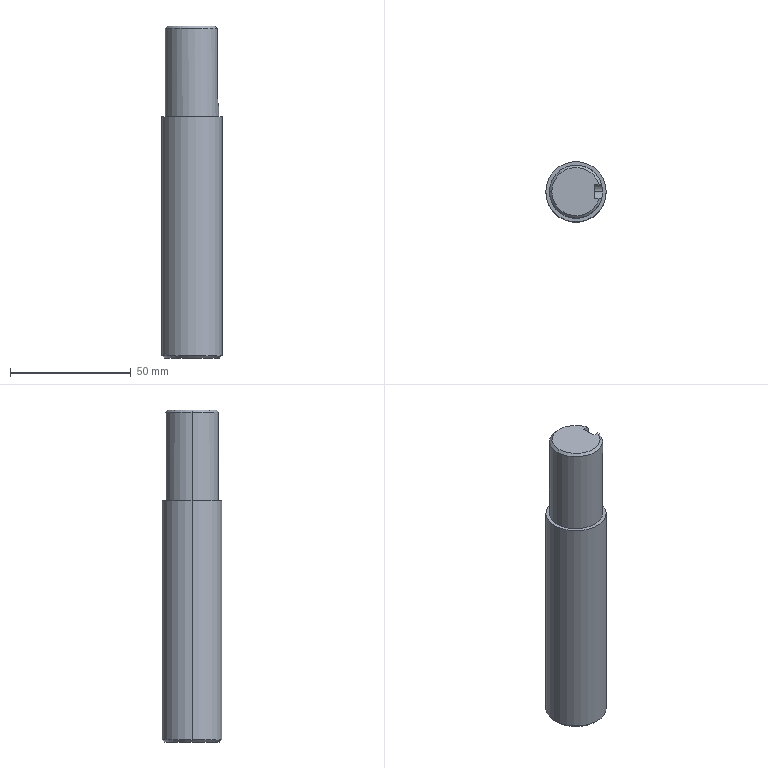Part | SolidWorks | features BaseBody 1 | 1 solid | 16 faces | box 25 x 25 x 137.5 mm | volume 62620 mm3 | cylinder 6 | plane 6 | cone 4 | commonest cylinder face diameters 6 x2 22 x2 25 x2
STEP:
#1=CARTESIAN_POINT('',(-12.5,0.,100.));
#2=VERTEX_POINT('',#1);
#3=CARTESIAN_POINT('',(12.5,0.,100.));
#4=VERTEX_POINT('',#3);
#5=CARTESIAN_POINT('',(0.,0.,100.));
#6=DIRECTION('',(0.,0.,-1.));
#7=DIRECTION('',(-1.,0.,0.));
#8=AXIS2_PLACEMENT_3D('',#5,#6,#7);
#9=CIRCLE('',#8,12.5);
#10=EDGE_CURVE('',#2,#4,#9,.T.);
#11=ORIENTED_EDGE('',*,*,#10,.T.);
#12=CARTESIAN_POINT('',(12.5,0.,1.));
#13=VERTEX_POINT('',#12);
#14=CARTESIAN_POINT('',(12.5,0.,100.));
#15=DIRECTION('',(0.,0.,-1.));
#16=VECTOR('',#15,1000.);
#17=LINE('',#14,#16);
#18=EDGE_CURVE('',#4,#13,#17,.T.);
#19=ORIENTED_EDGE('',*,*,#18,.T.);
#20=CARTESIAN_POINT('',(-12.5,0.,1.));
#21=VERTEX_POINT('',#20);
#22=CARTESIAN_POINT('',(0.,0.,1.));
#23=DIRECTION('',(0.,0.,1.));
#24=DIRECTION('',(-1.,0.,0.));
#25=AXIS2_PLACEMENT_3D('',#22,#23,#24);
#26=CIRCLE('',#25,12.5);
#27=EDGE_CURVE('',#13,#21,#26,.T.);
#28=ORIENTED_EDGE('',*,*,#27,.T.);
#29=CARTESIAN_POINT('',(-12.5,0.,100.));
#30=DIRECTION('',(0.,0.,-1.));
#31=VECTOR('',#30,1000.);
#32=LINE('',#29,#31);
#33=EDGE_CURVE('',#2,#21,#32,.T.);
#34=ORIENTED_EDGE('',*,*,#33,.F.);
#35=EDGE_LOOP('',(#11,#19,#28,#34));
#36=FACE_OUTER_BOUND('',#35,.T.);
#37=CARTESIAN_POINT('',(0.,0.,100.));
#38=DIRECTION('',(0.,0.,-1.));
#39=DIRECTION('',(-1.,0.,0.));
#40=AXIS2_PLACEMENT_3D('',#37,#38,#39);
#41=CYLINDRICAL_SURFACE('',#40,12.5);
#42=ADVANCED_FACE('',(#36),#41,.T.);
#43=CARTESIAN_POINT('',(11.5,0.,0.));
#44=VERTEX_POINT('',#43);
#45=CARTESIAN_POINT('',(-11.5,0.,0.));
#46=VERTEX_POINT('',#45);
#47=CARTESIAN_POINT('',(0.,0.,0.));
#48=DIRECTION('',(0.,0.,1.));
#49=DIRECTION('',(1.,0.,0.));
#50=AXIS2_PLACEMENT_3D('',#47,#48,#49);
#51=CIRCLE('',#50,11.5);
#52=EDGE_CURVE('',#44,#46,#51,.T.);
#53=ORIENTED_EDGE('',*,*,#52,.T.);
#54=CARTESIAN_POINT('',(-12.5,0.,1.));
#55=DIRECTION('',(-0.7071,0.,0.7071));
#56=VECTOR('',#55,1000.);
#57=LINE('',#54,#56);
#58=EDGE_CURVE('',#46,#21,#57,.T.);
#59=ORIENTED_EDGE('',*,*,#58,.T.);
#60=ORIENTED_EDGE('',*,*,#27,.F.);
#61=CARTESIAN_POINT('',(12.5,0.,1.));
#62=DIRECTION('',(0.7071,0.,0.7071));
#63=VECTOR('',#62,1000.);
#64=LINE('',#61,#63);
#65=EDGE_CURVE('',#44,#13,#64,.T.);
#66=ORIENTED_EDGE('',*,*,#65,.F.);
#67=EDGE_LOOP('',(#53,#59,#60,#66));
#68=FACE_OUTER_BOUND('',#67,.T.);
#69=CARTESIAN_POINT('',(0.,0.,1.));
#70=DIRECTION('',(0.,0.,1.));
#71=DIRECTION('',(1.,0.,0.));
#72=AXIS2_PLACEMENT_3D('',#69,#70,#71);
#73=CONICAL_SURFACE('',#72,12.5,0.7854);
#74=ADVANCED_FACE('',(#68),#73,.T.);
#75=CARTESIAN_POINT('',(10.583,3.,107.5));
#76=VERTEX_POINT('',#75);
#77=CARTESIAN_POINT('',(11.,0.,104.5));
#78=VERTEX_POINT('',#77);
#79=CARTESIAN_POINT('',(10.583,3.,107.5));
#80=CARTESIAN_POINT('',(10.583,3.,107.301));
#81=CARTESIAN_POINT('',(10.589,2.98,107.105));
#82=CARTESIAN_POINT('',(10.61,2.904,106.721));
#83=CARTESIAN_POINT('',(10.626,2.846,106.53));
#84=CARTESIAN_POINT('',(10.665,2.695,106.167));
#85=CARTESIAN_POINT('',(10.688,2.603,105.995));
#86=CARTESIAN_POINT('',(10.739,2.385,105.67));
#87=CARTESIAN_POINT('',(10.766,2.259,105.517));
#88=CARTESIAN_POINT('',(10.82,1.984,105.242));
#89=CARTESIAN_POINT('',(10.847,1.834,105.118));
#90=CARTESIAN_POINT('',(10.898,1.507,104.898));
#91=CARTESIAN_POINT('',(10.92,1.334,104.806));
#92=CARTESIAN_POINT('',(10.958,0.9736,104.656));
#93=CARTESIAN_POINT('',(10.974,0.784,104.597));
#94=CARTESIAN_POINT('',(10.995,0.3957,104.52));
#95=CARTESIAN_POINT('',(11.,0.1991,104.5));
#96=CARTESIAN_POINT('',(11.,0.,104.5));
#97=B_SPLINE_CURVE_WITH_KNOTS('',3,(#79,#80,#81,#82,#83,#84,#85,#86,#87,#88,#89,#90,#91,#92,#93,#94,#95,#96),.UNSPECIFIED.,.F.,.F.,(4,2,2,2,2,2,2,2,4),(0.,0.0005886,0.001177,0.001766,0.002354,0.002943,0.003532,0.00412,0.004709),.UNSPECIFIED.);
#98=EDGE_CURVE('',#76,#78,#97,.T.);
#99=ORIENTED_EDGE('',*,*,#98,.T.);
#100=CARTESIAN_POINT('',(11.,0.,100.));
#101=VERTEX_POINT('',#100);
#102=CARTESIAN_POINT('',(11.,0.,137.5));
#103=DIRECTION('',(0.,0.,-1.));
#104=VECTOR('',#103,1000.);
#105=LINE('',#102,#104);
#106=EDGE_CURVE('',#78,#101,#105,.T.);
#107=ORIENTED_EDGE('',*,*,#106,.T.);
#108=CARTESIAN_POINT('',(-11.,0.,100.));
#109=VERTEX_POINT('',#108);
#110=CARTESIAN_POINT('',(0.,0.,100.));
#111=DIRECTION('',(0.,0.,-1.));
#112=DIRECTION('',(-1.,0.,0.));
#113=AXIS2_PLACEMENT_3D('',#110,#111,#112);
#114=CIRCLE('',#113,11.);
#115=EDGE_CURVE('',#109,#101,#114,.T.);
#116=ORIENTED_EDGE('',*,*,#115,.F.);
#117=CARTESIAN_POINT('',(-11.,0.,136.5));
#118=VERTEX_POINT('',#117);
#119=CARTESIAN_POINT('',(-11.,0.,137.5));
#120=DIRECTION('',(0.,0.,-1.));
#121=VECTOR('',#120,1000.);
#122=LINE('',#119,#121);
#123=EDGE_CURVE('',#118,#109,#122,.T.);
#124=ORIENTED_EDGE('',*,*,#123,.F.);
#125=CARTESIAN_POINT('',(10.583,3.,136.5));
#126=VERTEX_POINT('',#125);
#127=CARTESIAN_POINT('',(0.,0.,136.5));
#128=DIRECTION('',(0.,0.,-1.));
#129=DIRECTION('',(-1.,0.,0.));
#130=AXIS2_PLACEMENT_3D('',#127,#128,#129);
#131=CIRCLE('',#130,11.);
#132=EDGE_CURVE('',#118,#126,#131,.T.);
#133=ORIENTED_EDGE('',*,*,#132,.T.);
#134=CARTESIAN_POINT('',(10.583,3.,137.5));
#135=DIRECTION('',(0.,0.,-1.));
#136=VECTOR('',#135,1000.);
#137=LINE('',#134,#136);
#138=EDGE_CURVE('',#126,#76,#137,.T.);
#139=ORIENTED_EDGE('',*,*,#138,.T.);
#140=EDGE_LOOP('',(#99,#107,#116,#124,#133,#139));
#141=FACE_OUTER_BOUND('',#140,.T.);
#142=CARTESIAN_POINT('',(0.,0.,137.5));
#143=DIRECTION('',(0.,0.,-1.));
#144=DIRECTION('',(-1.,0.,0.));
#145=AXIS2_PLACEMENT_3D('',#142,#143,#144);
#146=CYLINDRICAL_SURFACE('',#145,11.);
#147=ADVANCED_FACE('',(#141),#146,.T.);
#148=CARTESIAN_POINT('',(9.539,-3.,137.5));
#149=VERTEX_POINT('',#148);
#150=CARTESIAN_POINT('',(-10.,0.,137.5));
#151=VERTEX_POINT('',#150);
#152=CARTESIAN_POINT('',(0.,0.,137.5));
#153=DIRECTION('',(0.,0.,-1.));
#154=DIRECTION('',(-1.,0.,0.));
#155=AXIS2_PLACEMENT_3D('',#152,#153,#154);
#156=CIRCLE('',#155,10.);
#157=EDGE_CURVE('',#149,#151,#156,.T.);
#158=ORIENTED_EDGE('',*,*,#157,.T.);
#159=CARTESIAN_POINT('',(-11.,0.,136.5));
#160=DIRECTION('',(-0.7071,0.,-0.7071));
#161=VECTOR('',#160,1000.);
#162=LINE('',#159,#161);
#163=EDGE_CURVE('',#151,#118,#162,.T.);
#164=ORIENTED_EDGE('',*,*,#163,.T.);
#165=CARTESIAN_POINT('',(10.583,-3.,136.5));
#166=VERTEX_POINT('',#165);
#167=CARTESIAN_POINT('',(0.,0.,136.5));
#168=DIRECTION('',(0.,0.,-1.));
#169=DIRECTION('',(-1.,0.,0.));
#170=AXIS2_PLACEMENT_3D('',#167,#168,#169);
#171=CIRCLE('',#170,11.);
#172=EDGE_CURVE('',#166,#118,#171,.T.);
#173=ORIENTED_EDGE('',*,*,#172,.F.);
#174=CARTESIAN_POINT('',(10.583,-3.,136.5));
#175=CARTESIAN_POINT('',(10.236,-3.,136.834));
#176=CARTESIAN_POINT('',(9.888,-3.,137.167));
#177=CARTESIAN_POINT('',(9.539,-3.,137.5));
#178=B_SPLINE_CURVE_WITH_KNOTS('',3,(#174,#175,#176,#177),.UNSPECIFIED.,.F.,.F.,(4,4),(0.,0.001445),.UNSPECIFIED.);
#179=EDGE_CURVE('',#166,#149,#178,.T.);
#180=ORIENTED_EDGE('',*,*,#179,.T.);
#181=EDGE_LOOP('',(#158,#164,#173,#180));
#182=FACE_OUTER_BOUND('',#181,.T.);
#183=CARTESIAN_POINT('',(0.,0.,136.5));
#184=DIRECTION('',(0.,0.,-1.));
#185=DIRECTION('',(-1.,0.,0.));
#186=AXIS2_PLACEMENT_3D('',#183,#184,#185);
#187=CONICAL_SURFACE('',#186,11.,0.7854);
#188=ADVANCED_FACE('',(#182),#187,.T.);
#189=CARTESIAN_POINT('',(7.5,0.,104.5));
#190=VERTEX_POINT('',#189);
#191=CARTESIAN_POINT('',(7.5,3.,107.5));
#192=VERTEX_POINT('',#191);
#193=CARTESIAN_POINT('',(7.5,0.,107.5));
#194=DIRECTION('',(1.,0.,0.));
#195=DIRECTION('',(0.,0.,-1.));
#196=AXIS2_PLACEMENT_3D('',#193,#194,#195);
#197=CIRCLE('',#196,3.);
#198=EDGE_CURVE('',#190,#192,#197,.T.);
#199=ORIENTED_EDGE('',*,*,#198,.F.);
#200=CARTESIAN_POINT('',(7.5,0.,104.5));
#201=DIRECTION('',(1.,0.,0.));
#202=VECTOR('',#201,1000.);
#203=LINE('',#200,#202);
#204=EDGE_CURVE('',#190,#78,#203,.T.);
#205=ORIENTED_EDGE('',*,*,#204,.T.);
#206=ORIENTED_EDGE('',*,*,#98,.F.);
#207=CARTESIAN_POINT('',(7.5,3.,107.5));
#208=DIRECTION('',(-1.,0.,0.));
#209=VECTOR('',#208,1000.);
#210=LINE('',#207,#209);
#211=EDGE_CURVE('',#76,#192,#210,.T.);
#212=ORIENTED_EDGE('',*,*,#211,.T.);
#213=EDGE_LOOP('',(#199,#205,#206,#212));
#214=FACE_OUTER_BOUND('',#213,.T.);
#215=CARTESIAN_POINT('',(7.5,0.,107.5));
#216=DIRECTION('',(1.,0.,0.));
#217=DIRECTION('',(0.,0.,-1.));
#218=AXIS2_PLACEMENT_3D('',#215,#216,#217);
#219=CYLINDRICAL_SURFACE('',#218,3.);
#220=ADVANCED_FACE('',(#214),#219,.F.);
#221=ORIENTED_EDGE('',*,*,#18,.F.);
#222=CARTESIAN_POINT('',(0.,0.,100.));
#223=DIRECTION('',(0.,0.,-1.));
#224=DIRECTION('',(-1.,0.,0.));
#225=AXIS2_PLACEMENT_3D('',#222,#223,#224);
#226=CIRCLE('',#225,12.5);
#227=EDGE_CURVE('',#4,#2,#226,.T.);
#228=ORIENTED_EDGE('',*,*,#227,.T.);
#229=ORIENTED_EDGE('',*,*,#33,.T.);
#230=CARTESIAN_POINT('',(0.,0.,1.));
#231=DIRECTION('',(0.,0.,1.));
#232=DIRECTION('',(-1.,0.,0.));
#233=AXIS2_PLACEMENT_3D('',#230,#231,#232);
#234=CIRCLE('',#233,12.5);
#235=EDGE_CURVE('',#21,#13,#234,.T.);
#236=ORIENTED_EDGE('',*,*,#235,.T.);
#237=EDGE_LOOP('',(#221,#228,#229,#236));
#238=FACE_OUTER_BOUND('',#237,.T.);
#239=CARTESIAN_POINT('',(0.,0.,100.));
#240=DIRECTION('',(0.,0.,-1.));
#241=DIRECTION('',(-1.,0.,0.));
#242=AXIS2_PLACEMENT_3D('',#239,#240,#241);
#243=CYLINDRICAL_SURFACE('',#242,12.5);
#244=ADVANCED_FACE('',(#238),#243,.T.);
#245=ORIENTED_EDGE('',*,*,#58,.F.);
#246=CARTESIAN_POINT('',(0.,0.,0.));
#247=DIRECTION('',(0.,0.,1.));
#248=DIRECTION('',(1.,0.,0.));
#249=AXIS2_PLACEMENT_3D('',#246,#247,#248);
#250=CIRCLE('',#249,11.5);
#251=EDGE_CURVE('',#46,#44,#250,.T.);
#252=ORIENTED_EDGE('',*,*,#251,.T.);
#253=ORIENTED_EDGE('',*,*,#65,.T.);
#254=ORIENTED_EDGE('',*,*,#235,.F.);
#255=EDGE_LOOP('',(#245,#252,#253,#254));
#256=FACE_OUTER_BOUND('',#255,.T.);
#257=CARTESIAN_POINT('',(0.,0.,1.));
#258=DIRECTION('',(0.,0.,1.));
#259=DIRECTION('',(1.,0.,0.));
#260=AXIS2_PLACEMENT_3D('',#257,#258,#259);
#261=CONICAL_SURFACE('',#260,12.5,0.7854);
#262=ADVANCED_FACE('',(#256),#261,.T.);
#263=ORIENTED_EDGE('',*,*,#10,.F.);
#264=ORIENTED_EDGE('',*,*,#227,.F.);
#265=EDGE_LOOP('',(#263,#264));
#266=FACE_OUTER_BOUND('',#265,.T.);
#267=ORIENTED_EDGE('',*,*,#115,.T.);
#268=CARTESIAN_POINT('',(0.,0.,100.));
#269=DIRECTION('',(0.,0.,-1.));
#270=DIRECTION('',(-1.,0.,0.));
#271=AXIS2_PLACEMENT_3D('',#268,#269,#270);
#272=CIRCLE('',#271,11.);
#273=EDGE_CURVE('',#101,#109,#272,.T.);
#274=ORIENTED_EDGE('',*,*,#273,.T.);
#275=EDGE_LOOP('',(#267,#274));
#276=FACE_BOUND('',#275,.T.);
#277=CARTESIAN_POINT('',(0.,0.,100.));
#278=DIRECTION('',(0.,0.,1.));
#279=DIRECTION('',(1.,0.,0.));
#280=AXIS2_PLACEMENT_3D('',#277,#278,#279);
#281=PLANE('',#280);
#282=ADVANCED_FACE('',(#266,#276),#281,.T.);
#283=ORIENTED_EDGE('',*,*,#52,.F.);
#284=ORIENTED_EDGE('',*,*,#251,.F.);
#285=EDGE_LOOP('',(#283,#284));
#286=FACE_OUTER_BOUND('',#285,.T.);
#287=CARTESIAN_POINT('',(0.,0.,0.));
#288=DIRECTION('',(0.,0.,1.));
#289=DIRECTION('',(1.,0.,0.));
#290=AXIS2_PLACEMENT_3D('',#287,#288,#289);
#291=PLANE('',#290);
#292=ADVANCED_FACE('',(#286),#291,.F.);
#293=ORIENTED_EDGE('',*,*,#106,.F.);
#294=CARTESIAN_POINT('',(10.583,-3.,107.5));
#295=VERTEX_POINT('',#294);
#296=CARTESIAN_POINT('',(11.,0.,104.5));
#297=CARTESIAN_POINT('',(11.,-0.1991,104.5));
#298=CARTESIAN_POINT('',(10.995,-0.3947,104.52));
#299=CARTESIAN_POINT('',(10.974,-0.7792,104.596));
#300=CARTESIAN_POINT('',(10.959,-0.9702,104.654));
#301=CARTESIAN_POINT('',(10.92,-1.333,104.805));
#302=CARTESIAN_POINT('',(10.898,-1.505,104.897));
#303=CARTESIAN_POINT('',(10.848,-1.83,105.115));
#304=CARTESIAN_POINT('',(10.821,-1.983,105.241));
#305=CARTESIAN_POINT('',(10.767,-2.259,105.516));
#306=CARTESIAN_POINT('',(10.74,-2.382,105.666));
#307=CARTESIAN_POINT('',(10.688,-2.602,105.993));
#308=CARTESIAN_POINT('',(10.665,-2.694,106.166));
#309=CARTESIAN_POINT('',(10.626,-2.844,106.527));
#310=CARTESIAN_POINT('',(10.61,-2.903,106.716));
#311=CARTESIAN_POINT('',(10.589,-2.98,107.104));
#312=CARTESIAN_POINT('',(10.583,-3.,107.301));
#313=CARTESIAN_POINT('',(10.583,-3.,107.5));
#314=B_SPLINE_CURVE_WITH_KNOTS('',3,(#296,#297,#298,#299,#300,#301,#302,#303,#304,#305,#306,#307,#308,#309,#310,#311,#312,#313),.UNSPECIFIED.,.F.,.F.,(4,2,2,2,2,2,2,2,4),(0.004709,0.005298,0.005886,0.006475,0.007063,0.007652,0.008241,0.008829,0.009418),.UNSPECIFIED.);
#315=EDGE_CURVE('',#78,#295,#314,.T.);
#316=ORIENTED_EDGE('',*,*,#315,.T.);
#317=CARTESIAN_POINT('',(10.583,-3.,137.5));
#318=DIRECTION('',(0.,0.,1.));
#319=VECTOR('',#318,1000.);
#320=LINE('',#317,#319);
#321=EDGE_CURVE('',#295,#166,#320,.T.);
#322=ORIENTED_EDGE('',*,*,#321,.T.);
#323=ORIENTED_EDGE('',*,*,#172,.T.);
#324=ORIENTED_EDGE('',*,*,#123,.T.);
#325=ORIENTED_EDGE('',*,*,#273,.F.);
#326=EDGE_LOOP('',(#293,#316,#322,#323,#324,#325));
#327=FACE_OUTER_BOUND('',#326,.T.);
#328=CARTESIAN_POINT('',(0.,0.,137.5));
#329=DIRECTION('',(0.,0.,-1.));
#330=DIRECTION('',(-1.,0.,0.));
#331=AXIS2_PLACEMENT_3D('',#328,#329,#330);
#332=CYLINDRICAL_SURFACE('',#331,11.);
#333=ADVANCED_FACE('',(#327),#332,.T.);
#334=CARTESIAN_POINT('',(9.539,3.,137.5));
#335=VERTEX_POINT('',#334);
#336=CARTESIAN_POINT('',(9.539,3.,137.5));
#337=CARTESIAN_POINT('',(9.888,3.,137.167));
#338=CARTESIAN_POINT('',(10.236,3.,136.834));
#339=CARTESIAN_POINT('',(10.583,3.,136.5));
#340=B_SPLINE_CURVE_WITH_KNOTS('',3,(#336,#337,#338,#339),.UNSPECIFIED.,.F.,.F.,(4,4),(0.,0.001445),.UNSPECIFIED.);
#341=EDGE_CURVE('',#335,#126,#340,.T.);
#342=ORIENTED_EDGE('',*,*,#341,.F.);
#343=CARTESIAN_POINT('',(7.5,3.,137.5));
#344=VERTEX_POINT('',#343);
#345=CARTESIAN_POINT('',(7.5,3.,137.5));
#346=DIRECTION('',(1.,0.,0.));
#347=VECTOR('',#346,1000.);
#348=LINE('',#345,#347);
#349=EDGE_CURVE('',#344,#335,#348,.T.);
#350=ORIENTED_EDGE('',*,*,#349,.F.);
#351=CARTESIAN_POINT('',(7.5,3.,137.5));
#352=DIRECTION('',(0.,0.,1.));
#353=VECTOR('',#352,1000.);
#354=LINE('',#351,#353);
#355=EDGE_CURVE('',#192,#344,#354,.T.);
#356=ORIENTED_EDGE('',*,*,#355,.F.);
#357=ORIENTED_EDGE('',*,*,#211,.F.);
#358=ORIENTED_EDGE('',*,*,#138,.F.);
#359=EDGE_LOOP('',(#342,#350,#356,#357,#358));
#360=FACE_OUTER_BOUND('',#359,.T.);
#361=CARTESIAN_POINT('',(7.5,3.,137.5));
#362=DIRECTION('',(0.,1.,0.));
#363=DIRECTION('',(0.,0.,1.));
#364=AXIS2_PLACEMENT_3D('',#361,#362,#363);
#365=PLANE('',#364);
#366=ADVANCED_FACE('',(#360),#365,.F.);
#367=ORIENTED_EDGE('',*,*,#163,.F.);
#368=CARTESIAN_POINT('',(0.,0.,137.5));
#369=DIRECTION('',(0.,0.,-1.));
#370=DIRECTION('',(-1.,0.,0.));
#371=AXIS2_PLACEMENT_3D('',#368,#369,#370);
#372=CIRCLE('',#371,10.);
#373=EDGE_CURVE('',#151,#335,#372,.T.);
#374=ORIENTED_EDGE('',*,*,#373,.T.);
#375=ORIENTED_EDGE('',*,*,#341,.T.);
#376=ORIENTED_EDGE('',*,*,#132,.F.);
#377=EDGE_LOOP('',(#367,#374,#375,#376));
#378=FACE_OUTER_BOUND('',#377,.T.);
#379=CARTESIAN_POINT('',(0.,0.,136.5));
#380=DIRECTION('',(0.,0.,-1.));
#381=DIRECTION('',(-1.,0.,0.));
#382=AXIS2_PLACEMENT_3D('',#379,#380,#381);
#383=CONICAL_SURFACE('',#382,11.,0.7854);
#384=ADVANCED_FACE('',(#378),#383,.T.);
#385=ORIENTED_EDGE('',*,*,#204,.F.);
#386=CARTESIAN_POINT('',(7.5,-3.,107.5));
#387=VERTEX_POINT('',#386);
#388=CARTESIAN_POINT('',(7.5,0.,107.5));
#389=DIRECTION('',(1.,0.,0.));
#390=DIRECTION('',(0.,0.,-1.));
#391=AXIS2_PLACEMENT_3D('',#388,#389,#390);
#392=CIRCLE('',#391,3.);
#393=EDGE_CURVE('',#387,#190,#392,.T.);
#394=ORIENTED_EDGE('',*,*,#393,.F.);
#395=CARTESIAN_POINT('',(7.5,-3.,107.5));
#396=DIRECTION('',(1.,0.,0.));
#397=VECTOR('',#396,1000.);
#398=LINE('',#395,#397);
#399=EDGE_CURVE('',#387,#295,#398,.T.);
#400=ORIENTED_EDGE('',*,*,#399,.T.);
#401=ORIENTED_EDGE('',*,*,#315,.F.);
#402=EDGE_LOOP('',(#385,#394,#400,#401));
#403=FACE_OUTER_BOUND('',#402,.T.);
#404=CARTESIAN_POINT('',(7.5,0.,107.5));
#405=DIRECTION('',(1.,0.,0.));
#406=DIRECTION('',(0.,0.,-1.));
#407=AXIS2_PLACEMENT_3D('',#404,#405,#406);
#408=CYLINDRICAL_SURFACE('',#407,3.);
#409=ADVANCED_FACE('',(#403),#408,.F.);
#410=ORIENTED_EDGE('',*,*,#179,.F.);
#411=ORIENTED_EDGE('',*,*,#321,.F.);
#412=ORIENTED_EDGE('',*,*,#399,.F.);
#413=CARTESIAN_POINT('',(7.5,-3.,137.5));
#414=VERTEX_POINT('',#413);
#415=CARTESIAN_POINT('',(7.5,-3.,137.5));
#416=DIRECTION('',(0.,0.,-1.));
#417=VECTOR('',#416,1000.);
#418=LINE('',#415,#417);
#419=EDGE_CURVE('',#414,#387,#418,.T.);
#420=ORIENTED_EDGE('',*,*,#419,.F.);
#421=CARTESIAN_POINT('',(7.5,-3.,137.5));
#422=DIRECTION('',(-1.,0.,0.));
#423=VECTOR('',#422,1000.);
#424=LINE('',#421,#423);
#425=EDGE_CURVE('',#149,#414,#424,.T.);
#426=ORIENTED_EDGE('',*,*,#425,.F.);
#427=EDGE_LOOP('',(#410,#411,#412,#420,#426));
#428=FACE_OUTER_BOUND('',#427,.T.);
#429=CARTESIAN_POINT('',(7.5,-3.,137.5));
#430=DIRECTION('',(0.,-1.,0.));
#431=DIRECTION('',(0.,0.,-1.));
#432=AXIS2_PLACEMENT_3D('',#429,#430,#431);
#433=PLANE('',#432);
#434=ADVANCED_FACE('',(#428),#433,.F.);
#435=ORIENTED_EDGE('',*,*,#425,.T.);
#436=CARTESIAN_POINT('',(7.5,0.,137.5));
#437=DIRECTION('',(0.,1.,0.));
#438=VECTOR('',#437,1000.);
#439=LINE('',#436,#438);
#440=EDGE_CURVE('',#414,#344,#439,.T.);
#441=ORIENTED_EDGE('',*,*,#440,.T.);
#442=ORIENTED_EDGE('',*,*,#349,.T.);
#443=ORIENTED_EDGE('',*,*,#373,.F.);
#444=ORIENTED_EDGE('',*,*,#157,.F.);
#445=EDGE_LOOP('',(#435,#441,#442,#443,#444));
#446=FACE_OUTER_BOUND('',#445,.T.);
#447=CARTESIAN_POINT('',(0.,0.,137.5));
#448=DIRECTION('',(0.,0.,1.));
#449=DIRECTION('',(1.,0.,0.));
#450=AXIS2_PLACEMENT_3D('',#447,#448,#449);
#451=PLANE('',#450);
#452=ADVANCED_FACE('',(#446),#451,.T.);
#453=ORIENTED_EDGE('',*,*,#355,.T.);
#454=ORIENTED_EDGE('',*,*,#440,.F.);
#455=ORIENTED_EDGE('',*,*,#419,.T.);
#456=ORIENTED_EDGE('',*,*,#393,.T.);
#457=ORIENTED_EDGE('',*,*,#198,.T.);
#458=EDGE_LOOP('',(#453,#454,#455,#456,#457));
#459=FACE_OUTER_BOUND('',#458,.T.);
#460=CARTESIAN_POINT('',(7.5,0.,137.5));
#461=DIRECTION('',(1.,0.,0.));
#462=DIRECTION('',(0.,0.,-1.));
#463=AXIS2_PLACEMENT_3D('',#460,#461,#462);
#464=PLANE('',#463);
#465=ADVANCED_FACE('',(#459),#464,.T.);
#466=CLOSED_SHELL('',(#42,#74,#147,#188,#220,#244,#262,#282,#292,#333,#366,#384,#409,#434,#452,#465));
#467=MANIFOLD_SOLID_BREP('',#466);
#468=CARTESIAN_POINT('',(0.,0.,0.));
#469=DIRECTION('',(0.,0.,1.));
#470=DIRECTION('',(1.,0.,0.));
#471=AXIS2_PLACEMENT_3D('',#468,#469,#470);
#472=(LENGTH_UNIT()NAMED_UNIT(*)SI_UNIT(.MILLI.,.METRE.));
#473=UNCERTAINTY_MEASURE_WITH_UNIT(LENGTH_MEASURE(0.00001),#472,'','');
#474=(NAMED_UNIT(*)PLANE_ANGLE_UNIT()SI_UNIT($,.RADIAN.));
#475=(NAMED_UNIT(*)SI_UNIT($,.STERADIAN.)SOLID_ANGLE_UNIT());
#476=(GEOMETRIC_REPRESENTATION_CONTEXT(3)GLOBAL_UNCERTAINTY_ASSIGNED_CONTEXT((#473))GLOBAL_UNIT_ASSIGNED_CONTEXT((#472,#474,#475))REPRESENTATION_CONTEXT('',''));
#477=ADVANCED_BREP_SHAPE_REPRESENTATION('',(#467,#471),#476);